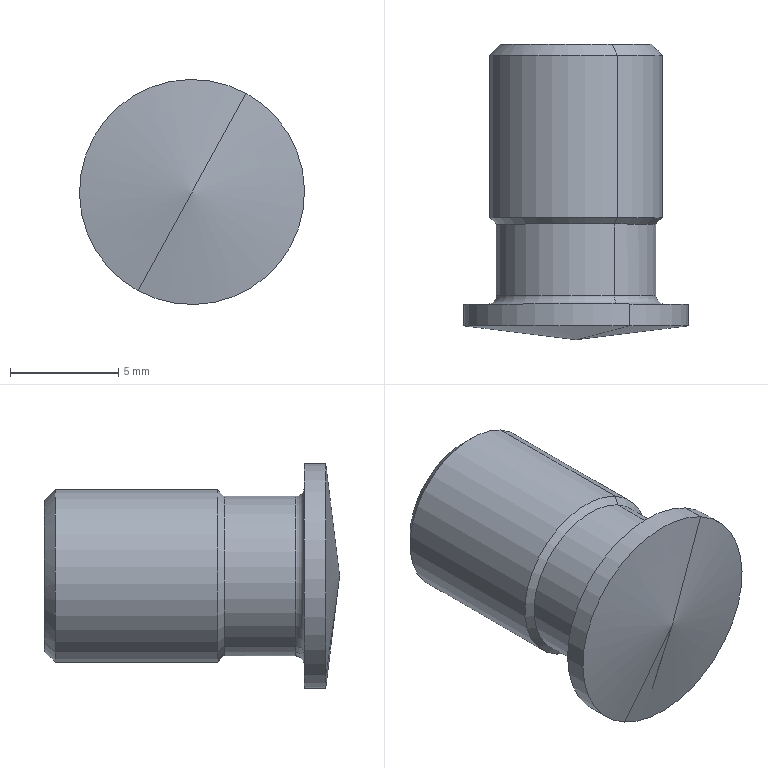Part | NX | features BREP 1 | 1 solid | 16 faces | box 10.4 x 13.638 x 10.4 mm | volume 676.067 mm3 | cone 6 | cylinder 6 | plane 2 | torus 2 | commonest cylinder face diameters 7.4 x2 8 x2 10.4 x2